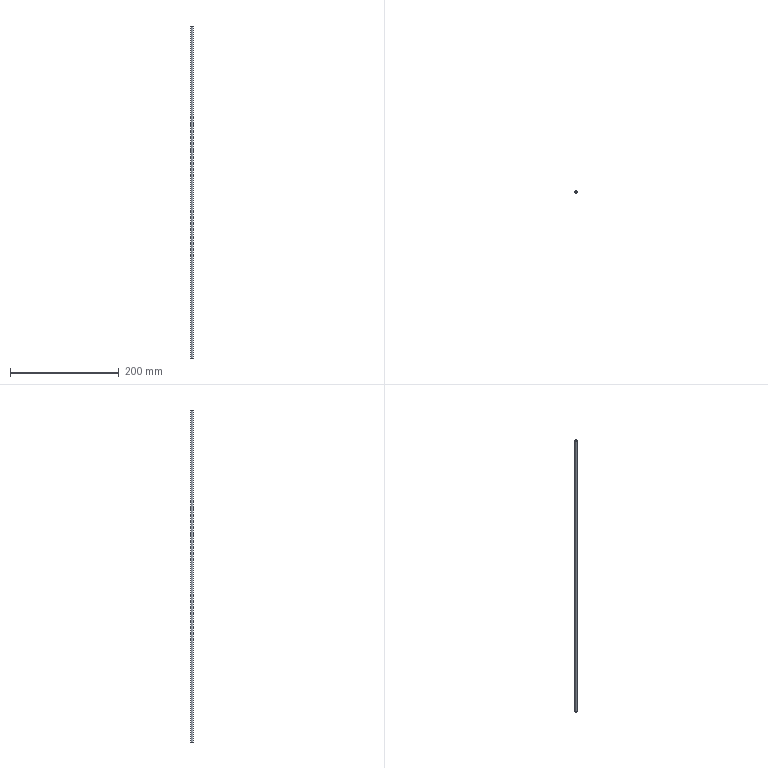Part | STEP file | JIS G 3191A - 6-1 | 1 solid | 3 faces | box 4 x 4 x 610 mm | volume 7665 mm3 | plane 2 | cylinder 1 | commonest cylinder face diameters 4 x1
STEP:
#1=CARTESIAN_POINT('',(0.,0.,0.));
#2=DIRECTION('',(0.,0.,1.));
#3=DIRECTION('',(1.,0.,0.));
#4=AXIS2_PLACEMENT_3D('',#1,#2,#3);
#5=CARTESIAN_POINT('',(2.,0.,610.));
#6=VERTEX_POINT('',#5);
#7=CARTESIAN_POINT('',(0.,0.,610.));
#8=DIRECTION('',(0.,0.,-1.));
#9=DIRECTION('',(-1.,0.,0.));
#10=AXIS2_PLACEMENT_3D('',#7,#8,#9);
#11=CIRCLE('',#10,2.);
#12=CARTESIAN_POINT('',(0.,0.,0.));
#13=DIRECTION('',(0.,0.,1.));
#14=DIRECTION('',(-1.,0.,0.));
#15=AXIS2_PLACEMENT_3D('',#12,#13,#14);
#16=CYLINDRICAL_SURFACE('',#15,2.);
#17=CARTESIAN_POINT('',(12.566,610.));
#18=DIRECTION('',(-1.,0.));
#19=VECTOR('',#18,1.);
#20=LINE('',#17,#19);
#21=(GEOMETRIC_REPRESENTATION_CONTEXT(2)PARAMETRIC_REPRESENTATION_CONTEXT()REPRESENTATION_CONTEXT('',''));
#22=DEFINITIONAL_REPRESENTATION('',(#20),#21);
#23=PCURVE('',#16,#22);
#24=CARTESIAN_POINT('',(0.,0.,610.));
#25=DIRECTION('',(0.,0.,1.));
#26=DIRECTION('',(1.,0.,0.));
#27=AXIS2_PLACEMENT_3D('',#24,#25,#26);
#28=PLANE('',#27);
#29=CARTESIAN_POINT('',(-2.,0.));
#30=CARTESIAN_POINT('',(-2.,3.464));
#31=CARTESIAN_POINT('',(1.,1.732));
#32=CARTESIAN_POINT('',(4.,0.));
#33=CARTESIAN_POINT('',(1.,-1.732));
#34=CARTESIAN_POINT('',(-2.,-3.464));
#35=CARTESIAN_POINT('',(-2.,0.));
#36=(BOUNDED_CURVE()B_SPLINE_CURVE(2,(#29,#30,#31,#32,#33,#34,#35),.UNSPECIFIED.,.T.,.F.)B_SPLINE_CURVE_WITH_KNOTS((1,2,2,2,2,1),(-2.094,0.,2.094,4.189,6.283,8.378),.UNSPECIFIED.)CURVE()GEOMETRIC_REPRESENTATION_ITEM()RATIONAL_B_SPLINE_CURVE((1.,0.5,1.,0.5,1.,0.5,1.))REPRESENTATION_ITEM(''));
#37=(GEOMETRIC_REPRESENTATION_CONTEXT(2)PARAMETRIC_REPRESENTATION_CONTEXT()REPRESENTATION_CONTEXT('',''));
#38=DEFINITIONAL_REPRESENTATION('',(#36),#37);
#39=PCURVE('',#28,#38);
#40=SURFACE_CURVE('',#11,(#23,#39),.PCURVE_S1.);
#41=EDGE_CURVE('',#6,#6,#40,.T.);
#42=ORIENTED_EDGE('',*,*,#41,.T.);
#43=CARTESIAN_POINT('',(2.,0.,0.));
#44=VERTEX_POINT('',#43);
#45=CARTESIAN_POINT('',(2.,0.,0.));
#46=CARTESIAN_POINT('',(2.,0.,610.));
#47=B_SPLINE_CURVE_WITH_KNOTS('',1,(#45,#46),.UNSPECIFIED.,.F.,.F.,(2,2),(0.,610.),.PIECEWISE_BEZIER_KNOTS.);
#48=CARTESIAN_POINT('',(3.142,0.));
#49=DIRECTION('',(0.,1.));
#50=VECTOR('',#49,1.);
#51=LINE('',#48,#50);
#52=(GEOMETRIC_REPRESENTATION_CONTEXT(2)PARAMETRIC_REPRESENTATION_CONTEXT()REPRESENTATION_CONTEXT('',''));
#53=DEFINITIONAL_REPRESENTATION('',(#51),#52);
#54=PCURVE('',#16,#53);
#55=CARTESIAN_POINT('',(9.425,0.));
#56=DIRECTION('',(0.,1.));
#57=VECTOR('',#56,1.);
#58=LINE('',#55,#57);
#59=(GEOMETRIC_REPRESENTATION_CONTEXT(2)PARAMETRIC_REPRESENTATION_CONTEXT()REPRESENTATION_CONTEXT('',''));
#60=DEFINITIONAL_REPRESENTATION('',(#58),#59);
#61=PCURVE('',#16,#60);
#62=SEAM_CURVE('',#47,(#54,#61),.PCURVE_S1.);
#63=EDGE_CURVE('',#44,#6,#62,.T.);
#64=ORIENTED_EDGE('',*,*,#63,.F.);
#65=CARTESIAN_POINT('',(0.,0.,0.));
#66=DIRECTION('',(0.,0.,-1.));
#67=DIRECTION('',(-1.,0.,0.));
#68=AXIS2_PLACEMENT_3D('',#65,#66,#67);
#69=CIRCLE('',#68,2.);
#70=CARTESIAN_POINT('',(12.566,0.));
#71=DIRECTION('',(-1.,0.));
#72=VECTOR('',#71,1.);
#73=LINE('',#70,#72);
#74=(GEOMETRIC_REPRESENTATION_CONTEXT(2)PARAMETRIC_REPRESENTATION_CONTEXT()REPRESENTATION_CONTEXT('',''));
#75=DEFINITIONAL_REPRESENTATION('',(#73),#74);
#76=PCURVE('',#16,#75);
#77=CARTESIAN_POINT('',(0.,0.,0.));
#78=DIRECTION('',(0.,0.,1.));
#79=DIRECTION('',(1.,0.,0.));
#80=AXIS2_PLACEMENT_3D('',#77,#78,#79);
#81=PLANE('',#80);
#82=CARTESIAN_POINT('',(-2.,0.));
#83=CARTESIAN_POINT('',(-2.,3.464));
#84=CARTESIAN_POINT('',(1.,1.732));
#85=CARTESIAN_POINT('',(4.,0.));
#86=CARTESIAN_POINT('',(1.,-1.732));
#87=CARTESIAN_POINT('',(-2.,-3.464));
#88=CARTESIAN_POINT('',(-2.,0.));
#89=(BOUNDED_CURVE()B_SPLINE_CURVE(2,(#82,#83,#84,#85,#86,#87,#88),.UNSPECIFIED.,.T.,.F.)B_SPLINE_CURVE_WITH_KNOTS((1,2,2,2,2,1),(-2.094,0.,2.094,4.189,6.283,8.378),.UNSPECIFIED.)CURVE()GEOMETRIC_REPRESENTATION_ITEM()RATIONAL_B_SPLINE_CURVE((1.,0.5,1.,0.5,1.,0.5,1.))REPRESENTATION_ITEM(''));
#90=(GEOMETRIC_REPRESENTATION_CONTEXT(2)PARAMETRIC_REPRESENTATION_CONTEXT()REPRESENTATION_CONTEXT('',''));
#91=DEFINITIONAL_REPRESENTATION('',(#89),#90);
#92=PCURVE('',#81,#91);
#93=SURFACE_CURVE('',#69,(#76,#92),.PCURVE_S1.);
#94=EDGE_CURVE('',#44,#44,#93,.T.);
#95=ORIENTED_EDGE('',*,*,#94,.F.);
#96=ORIENTED_EDGE('',*,*,#63,.T.);
#97=EDGE_LOOP('',(#42,#64,#95,#96));
#98=FACE_BOUND('',#97,.T.);
#99=ADVANCED_FACE('',(#98),#16,.T.);
#100=ORIENTED_EDGE('',*,*,#94,.T.);
#101=EDGE_LOOP('',(#100));
#102=FACE_BOUND('',#101,.T.);
#103=ADVANCED_FACE('',(#102),#81,.F.);
#104=ORIENTED_EDGE('',*,*,#41,.F.);
#105=EDGE_LOOP('',(#104));
#106=FACE_BOUND('',#105,.T.);
#107=ADVANCED_FACE('',(#106),#28,.T.);
#108=CLOSED_SHELL('',(#99,#103,#107));
#109=MANIFOLD_SOLID_BREP('',#108);
#110=(LENGTH_UNIT()NAMED_UNIT(*)SI_UNIT(.MILLI.,.METRE.));
#111=UNCERTAINTY_MEASURE_WITH_UNIT(LENGTH_MEASURE(0.00001),#110,'','');
#112=(NAMED_UNIT(*)PLANE_ANGLE_UNIT()SI_UNIT($,.RADIAN.));
#113=(NAMED_UNIT(*)SI_UNIT($,.STERADIAN.)SOLID_ANGLE_UNIT());
#114=(GEOMETRIC_REPRESENTATION_CONTEXT(3)GLOBAL_UNCERTAINTY_ASSIGNED_CONTEXT((#111))GLOBAL_UNIT_ASSIGNED_CONTEXT((#110,#112,#113))REPRESENTATION_CONTEXT('',''));
#115=ADVANCED_BREP_SHAPE_REPRESENTATION('',(#4,#109),#114);